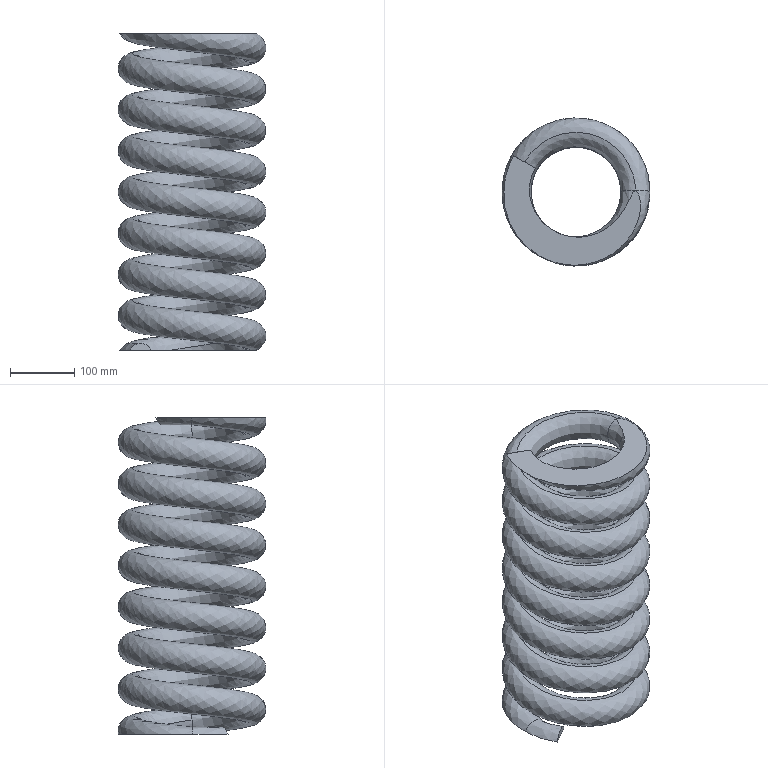Part | NX | features BREP 1 | 1 solid | 13 faces | volume 7127986 mm3 | spline 9 | plane 4